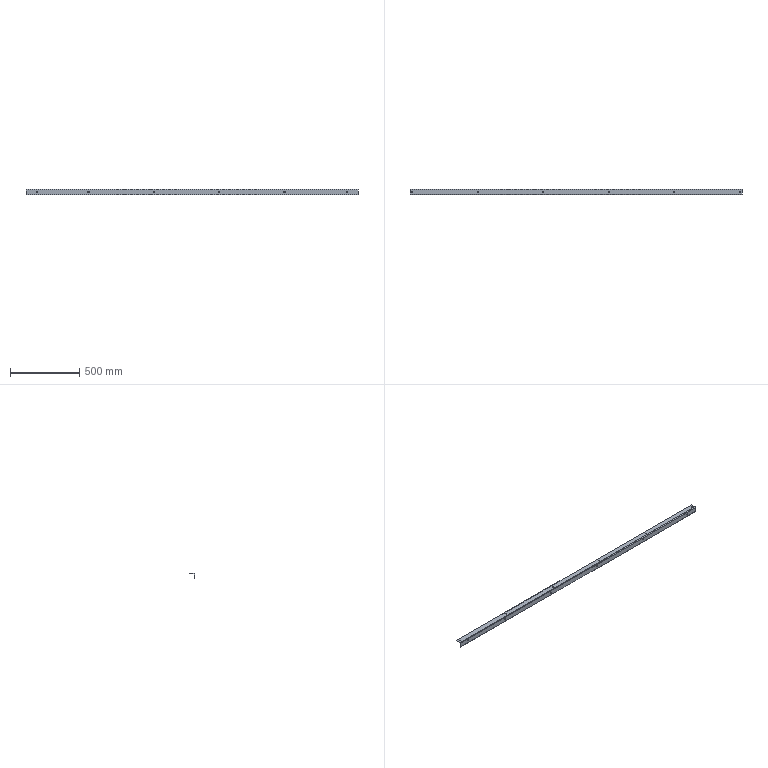Part | STEP file | 1 solid | 36 faces | box 2400 x 40 x 40 mm | volume 537626 mm3 | cylinder 28 | plane 8 | commonest cylinder face diameters 7 x12 9 x12 4 x3 10 x1